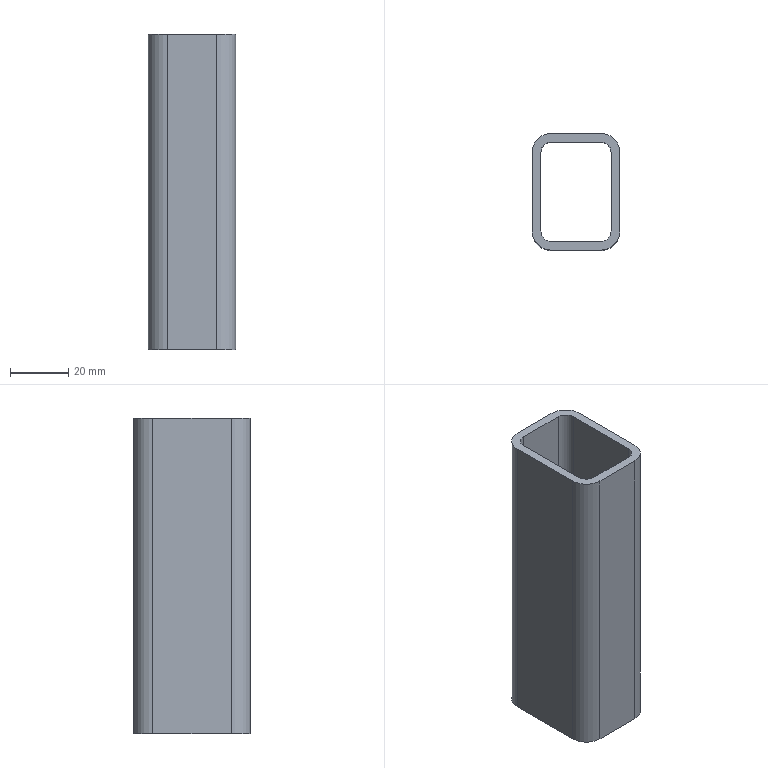Part | STEP file | DIN EN 10305-5 40 x 30 x 3 1785429742031 | 1 solid | 18 faces | box 30 x 40 x 108 mm | volume 38635 mm3 | plane 10 | cylinder 8 | commonest cylinder face diameters 7.2 x4 13.2 x4
STEP:
#1=CARTESIAN_POINT('',(-8.4,-17.,108.));
#2=VERTEX_POINT('',#1);
#3=CARTESIAN_POINT('',(8.4,-17.,108.));
#4=VERTEX_POINT('',#3);
#5=CARTESIAN_POINT('',(4.2,-17.,108.));
#6=DIRECTION('',(1.,0.,0.));
#7=VECTOR('',#6,10.);
#8=LINE('',#5,#7);
#9=EDGE_CURVE('',#2,#4,#8,.T.);
#10=ORIENTED_EDGE('',*,*,#9,.T.);
#11=CARTESIAN_POINT('',(8.4,-17.,0.));
#12=VERTEX_POINT('',#11);
#13=CARTESIAN_POINT('',(8.4,-17.,0.));
#14=DIRECTION('',(0.,0.,1.));
#15=VECTOR('',#14,10.);
#16=LINE('',#13,#15);
#17=EDGE_CURVE('',#12,#4,#16,.T.);
#18=ORIENTED_EDGE('',*,*,#17,.F.);
#19=CARTESIAN_POINT('',(-8.4,-17.,0.));
#20=VERTEX_POINT('',#19);
#21=CARTESIAN_POINT('',(4.2,-17.,0.));
#22=DIRECTION('',(1.,0.,0.));
#23=VECTOR('',#22,10.);
#24=LINE('',#21,#23);
#25=EDGE_CURVE('',#20,#12,#24,.T.);
#26=ORIENTED_EDGE('',*,*,#25,.F.);
#27=CARTESIAN_POINT('',(-8.4,-17.,0.));
#28=DIRECTION('',(0.,0.,1.));
#29=VECTOR('',#28,10.);
#30=LINE('',#27,#29);
#31=EDGE_CURVE('',#20,#2,#30,.T.);
#32=ORIENTED_EDGE('',*,*,#31,.T.);
#33=EDGE_LOOP('',(#10,#18,#26,#32));
#34=FACE_OUTER_BOUND('',#33,.T.);
#35=CARTESIAN_POINT('',(8.4,-17.,0.));
#36=DIRECTION('',(0.,-1.,0.));
#37=DIRECTION('',(0.,0.,-1.));
#38=AXIS2_PLACEMENT_3D('',#35,#36,#37);
#39=PLANE('',#38);
#40=ADVANCED_FACE('',(#34),#39,.F.);
#41=CARTESIAN_POINT('',(12.,-13.4,108.));
#42=VERTEX_POINT('',#41);
#43=CARTESIAN_POINT('',(8.4,-13.4,108.));
#44=DIRECTION('',(0.,0.,1.));
#45=DIRECTION('',(0.,1.,0.));
#46=AXIS2_PLACEMENT_3D('',#43,#44,#45);
#47=CIRCLE('',#46,3.6);
#48=EDGE_CURVE('',#4,#42,#47,.T.);
#49=ORIENTED_EDGE('',*,*,#48,.T.);
#50=CARTESIAN_POINT('',(12.,-13.4,0.));
#51=VERTEX_POINT('',#50);
#52=CARTESIAN_POINT('',(12.,-13.4,0.));
#53=DIRECTION('',(0.,0.,1.));
#54=VECTOR('',#53,10.);
#55=LINE('',#52,#54);
#56=EDGE_CURVE('',#51,#42,#55,.T.);
#57=ORIENTED_EDGE('',*,*,#56,.F.);
#58=CARTESIAN_POINT('',(8.4,-13.4,0.));
#59=DIRECTION('',(0.,0.,1.));
#60=DIRECTION('',(0.,1.,0.));
#61=AXIS2_PLACEMENT_3D('',#58,#59,#60);
#62=CIRCLE('',#61,3.6);
#63=EDGE_CURVE('',#12,#51,#62,.T.);
#64=ORIENTED_EDGE('',*,*,#63,.F.);
#65=ORIENTED_EDGE('',*,*,#17,.T.);
#66=EDGE_LOOP('',(#49,#57,#64,#65));
#67=FACE_OUTER_BOUND('',#66,.T.);
#68=CARTESIAN_POINT('',(8.4,-13.4,0.));
#69=DIRECTION('',(0.,0.,1.));
#70=DIRECTION('',(0.,1.,0.));
#71=AXIS2_PLACEMENT_3D('',#68,#69,#70);
#72=CYLINDRICAL_SURFACE('',#71,3.6);
#73=ADVANCED_FACE('',(#67),#72,.F.);
#74=CARTESIAN_POINT('',(12.,13.4,108.));
#75=VERTEX_POINT('',#74);
#76=CARTESIAN_POINT('',(12.,6.7,108.));
#77=DIRECTION('',(0.,1.,0.));
#78=VECTOR('',#77,10.);
#79=LINE('',#76,#78);
#80=EDGE_CURVE('',#42,#75,#79,.T.);
#81=ORIENTED_EDGE('',*,*,#80,.T.);
#82=CARTESIAN_POINT('',(12.,13.4,0.));
#83=VERTEX_POINT('',#82);
#84=CARTESIAN_POINT('',(12.,13.4,0.));
#85=DIRECTION('',(0.,0.,1.));
#86=VECTOR('',#85,10.);
#87=LINE('',#84,#86);
#88=EDGE_CURVE('',#83,#75,#87,.T.);
#89=ORIENTED_EDGE('',*,*,#88,.F.);
#90=CARTESIAN_POINT('',(12.,6.7,0.));
#91=DIRECTION('',(0.,1.,0.));
#92=VECTOR('',#91,10.);
#93=LINE('',#90,#92);
#94=EDGE_CURVE('',#51,#83,#93,.T.);
#95=ORIENTED_EDGE('',*,*,#94,.F.);
#96=ORIENTED_EDGE('',*,*,#56,.T.);
#97=EDGE_LOOP('',(#81,#89,#95,#96));
#98=FACE_OUTER_BOUND('',#97,.T.);
#99=CARTESIAN_POINT('',(12.,13.4,0.));
#100=DIRECTION('',(1.,0.,0.));
#101=DIRECTION('',(0.,0.,-1.));
#102=AXIS2_PLACEMENT_3D('',#99,#100,#101);
#103=PLANE('',#102);
#104=ADVANCED_FACE('',(#98),#103,.F.);
#105=CARTESIAN_POINT('',(8.4,17.,108.));
#106=VERTEX_POINT('',#105);
#107=CARTESIAN_POINT('',(8.4,13.4,108.));
#108=DIRECTION('',(0.,0.,1.));
#109=DIRECTION('',(-1.,0.,0.));
#110=AXIS2_PLACEMENT_3D('',#107,#108,#109);
#111=CIRCLE('',#110,3.6);
#112=EDGE_CURVE('',#75,#106,#111,.T.);
#113=ORIENTED_EDGE('',*,*,#112,.T.);
#114=CARTESIAN_POINT('',(8.4,17.,0.));
#115=VERTEX_POINT('',#114);
#116=CARTESIAN_POINT('',(8.4,17.,0.));
#117=DIRECTION('',(0.,0.,1.));
#118=VECTOR('',#117,10.);
#119=LINE('',#116,#118);
#120=EDGE_CURVE('',#115,#106,#119,.T.);
#121=ORIENTED_EDGE('',*,*,#120,.F.);
#122=CARTESIAN_POINT('',(8.4,13.4,0.));
#123=DIRECTION('',(0.,0.,1.));
#124=DIRECTION('',(-1.,0.,0.));
#125=AXIS2_PLACEMENT_3D('',#122,#123,#124);
#126=CIRCLE('',#125,3.6);
#127=EDGE_CURVE('',#83,#115,#126,.T.);
#128=ORIENTED_EDGE('',*,*,#127,.F.);
#129=ORIENTED_EDGE('',*,*,#88,.T.);
#130=EDGE_LOOP('',(#113,#121,#128,#129));
#131=FACE_OUTER_BOUND('',#130,.T.);
#132=CARTESIAN_POINT('',(8.4,13.4,0.));
#133=DIRECTION('',(0.,0.,1.));
#134=DIRECTION('',(-1.,0.,0.));
#135=AXIS2_PLACEMENT_3D('',#132,#133,#134);
#136=CYLINDRICAL_SURFACE('',#135,3.6);
#137=ADVANCED_FACE('',(#131),#136,.F.);
#138=CARTESIAN_POINT('',(15.,13.4,108.));
#139=VERTEX_POINT('',#138);
#140=CARTESIAN_POINT('',(15.,-13.4,108.));
#141=VERTEX_POINT('',#140);
#142=CARTESIAN_POINT('',(15.,6.7,108.));
#143=DIRECTION('',(0.,-1.,0.));
#144=VECTOR('',#143,10.);
#145=LINE('',#142,#144);
#146=EDGE_CURVE('',#139,#141,#145,.T.);
#147=ORIENTED_EDGE('',*,*,#146,.T.);
#148=CARTESIAN_POINT('',(15.,-13.4,0.));
#149=VERTEX_POINT('',#148);
#150=CARTESIAN_POINT('',(15.,-13.4,0.));
#151=DIRECTION('',(0.,0.,1.));
#152=VECTOR('',#151,10.);
#153=LINE('',#150,#152);
#154=EDGE_CURVE('',#149,#141,#153,.T.);
#155=ORIENTED_EDGE('',*,*,#154,.F.);
#156=CARTESIAN_POINT('',(15.,13.4,0.));
#157=VERTEX_POINT('',#156);
#158=CARTESIAN_POINT('',(15.,6.7,0.));
#159=DIRECTION('',(0.,-1.,0.));
#160=VECTOR('',#159,10.);
#161=LINE('',#158,#160);
#162=EDGE_CURVE('',#157,#149,#161,.T.);
#163=ORIENTED_EDGE('',*,*,#162,.F.);
#164=CARTESIAN_POINT('',(15.,13.4,0.));
#165=DIRECTION('',(0.,0.,1.));
#166=VECTOR('',#165,10.);
#167=LINE('',#164,#166);
#168=EDGE_CURVE('',#157,#139,#167,.T.);
#169=ORIENTED_EDGE('',*,*,#168,.T.);
#170=EDGE_LOOP('',(#147,#155,#163,#169));
#171=FACE_OUTER_BOUND('',#170,.T.);
#172=CARTESIAN_POINT('',(15.,13.4,0.));
#173=DIRECTION('',(1.,0.,0.));
#174=DIRECTION('',(0.,0.,-1.));
#175=AXIS2_PLACEMENT_3D('',#172,#173,#174);
#176=PLANE('',#175);
#177=ADVANCED_FACE('',(#171),#176,.T.);
#178=CARTESIAN_POINT('',(8.4,-20.,108.));
#179=VERTEX_POINT('',#178);
#180=CARTESIAN_POINT('',(8.4,-13.4,108.));
#181=DIRECTION('',(0.,0.,-1.));
#182=DIRECTION('',(0.,1.,0.));
#183=AXIS2_PLACEMENT_3D('',#180,#181,#182);
#184=CIRCLE('',#183,6.6);
#185=EDGE_CURVE('',#141,#179,#184,.T.);
#186=ORIENTED_EDGE('',*,*,#185,.T.);
#187=CARTESIAN_POINT('',(8.4,-20.,0.));
#188=VERTEX_POINT('',#187);
#189=CARTESIAN_POINT('',(8.4,-20.,0.));
#190=DIRECTION('',(0.,0.,1.));
#191=VECTOR('',#190,10.);
#192=LINE('',#189,#191);
#193=EDGE_CURVE('',#188,#179,#192,.T.);
#194=ORIENTED_EDGE('',*,*,#193,.F.);
#195=CARTESIAN_POINT('',(8.4,-13.4,0.));
#196=DIRECTION('',(0.,0.,-1.));
#197=DIRECTION('',(0.,1.,0.));
#198=AXIS2_PLACEMENT_3D('',#195,#196,#197);
#199=CIRCLE('',#198,6.6);
#200=EDGE_CURVE('',#149,#188,#199,.T.);
#201=ORIENTED_EDGE('',*,*,#200,.F.);
#202=ORIENTED_EDGE('',*,*,#154,.T.);
#203=EDGE_LOOP('',(#186,#194,#201,#202));
#204=FACE_OUTER_BOUND('',#203,.T.);
#205=CARTESIAN_POINT('',(8.4,-13.4,0.));
#206=DIRECTION('',(0.,0.,1.));
#207=DIRECTION('',(0.,1.,0.));
#208=AXIS2_PLACEMENT_3D('',#205,#206,#207);
#209=CYLINDRICAL_SURFACE('',#208,6.6);
#210=ADVANCED_FACE('',(#204),#209,.T.);
#211=CARTESIAN_POINT('',(-8.4,-20.,108.));
#212=VERTEX_POINT('',#211);
#213=CARTESIAN_POINT('',(4.2,-20.,108.));
#214=DIRECTION('',(-1.,0.,0.));
#215=VECTOR('',#214,10.);
#216=LINE('',#213,#215);
#217=EDGE_CURVE('',#179,#212,#216,.T.);
#218=ORIENTED_EDGE('',*,*,#217,.T.);
#219=CARTESIAN_POINT('',(-8.4,-20.,0.));
#220=VERTEX_POINT('',#219);
#221=CARTESIAN_POINT('',(-8.4,-20.,0.));
#222=DIRECTION('',(0.,0.,1.));
#223=VECTOR('',#222,10.);
#224=LINE('',#221,#223);
#225=EDGE_CURVE('',#220,#212,#224,.T.);
#226=ORIENTED_EDGE('',*,*,#225,.F.);
#227=CARTESIAN_POINT('',(4.2,-20.,0.));
#228=DIRECTION('',(-1.,0.,0.));
#229=VECTOR('',#228,10.);
#230=LINE('',#227,#229);
#231=EDGE_CURVE('',#188,#220,#230,.T.);
#232=ORIENTED_EDGE('',*,*,#231,.F.);
#233=ORIENTED_EDGE('',*,*,#193,.T.);
#234=EDGE_LOOP('',(#218,#226,#232,#233));
#235=FACE_OUTER_BOUND('',#234,.T.);
#236=CARTESIAN_POINT('',(8.4,-20.,0.));
#237=DIRECTION('',(0.,-1.,0.));
#238=DIRECTION('',(0.,0.,-1.));
#239=AXIS2_PLACEMENT_3D('',#236,#237,#238);
#240=PLANE('',#239);
#241=ADVANCED_FACE('',(#235),#240,.T.);
#242=CARTESIAN_POINT('',(-15.,-13.4,108.));
#243=VERTEX_POINT('',#242);
#244=CARTESIAN_POINT('',(-8.4,-13.4,108.));
#245=DIRECTION('',(0.,0.,-1.));
#246=DIRECTION('',(1.,0.,0.));
#247=AXIS2_PLACEMENT_3D('',#244,#245,#246);
#248=CIRCLE('',#247,6.6);
#249=EDGE_CURVE('',#212,#243,#248,.T.);
#250=ORIENTED_EDGE('',*,*,#249,.T.);
#251=CARTESIAN_POINT('',(-15.,-13.4,0.));
#252=VERTEX_POINT('',#251);
#253=CARTESIAN_POINT('',(-15.,-13.4,0.));
#254=DIRECTION('',(0.,0.,1.));
#255=VECTOR('',#254,10.);
#256=LINE('',#253,#255);
#257=EDGE_CURVE('',#252,#243,#256,.T.);
#258=ORIENTED_EDGE('',*,*,#257,.F.);
#259=CARTESIAN_POINT('',(-8.4,-13.4,0.));
#260=DIRECTION('',(0.,0.,-1.));
#261=DIRECTION('',(1.,0.,0.));
#262=AXIS2_PLACEMENT_3D('',#259,#260,#261);
#263=CIRCLE('',#262,6.6);
#264=EDGE_CURVE('',#220,#252,#263,.T.);
#265=ORIENTED_EDGE('',*,*,#264,.F.);
#266=ORIENTED_EDGE('',*,*,#225,.T.);
#267=EDGE_LOOP('',(#250,#258,#265,#266));
#268=FACE_OUTER_BOUND('',#267,.T.);
#269=CARTESIAN_POINT('',(-8.4,-13.4,0.));
#270=DIRECTION('',(0.,0.,1.));
#271=DIRECTION('',(1.,0.,0.));
#272=AXIS2_PLACEMENT_3D('',#269,#270,#271);
#273=CYLINDRICAL_SURFACE('',#272,6.6);
#274=ADVANCED_FACE('',(#268),#273,.T.);
#275=CARTESIAN_POINT('',(-8.4,17.,108.));
#276=VERTEX_POINT('',#275);
#277=CARTESIAN_POINT('',(-4.2,17.,108.));
#278=DIRECTION('',(-1.,0.,0.));
#279=VECTOR('',#278,10.);
#280=LINE('',#277,#279);
#281=EDGE_CURVE('',#106,#276,#280,.T.);
#282=ORIENTED_EDGE('',*,*,#281,.T.);
#283=CARTESIAN_POINT('',(-8.4,17.,0.));
#284=VERTEX_POINT('',#283);
#285=CARTESIAN_POINT('',(-8.4,17.,0.));
#286=DIRECTION('',(0.,0.,1.));
#287=VECTOR('',#286,10.);
#288=LINE('',#285,#287);
#289=EDGE_CURVE('',#284,#276,#288,.T.);
#290=ORIENTED_EDGE('',*,*,#289,.F.);
#291=CARTESIAN_POINT('',(-4.2,17.,0.));
#292=DIRECTION('',(-1.,0.,0.));
#293=VECTOR('',#292,10.);
#294=LINE('',#291,#293);
#295=EDGE_CURVE('',#115,#284,#294,.T.);
#296=ORIENTED_EDGE('',*,*,#295,.F.);
#297=ORIENTED_EDGE('',*,*,#120,.T.);
#298=EDGE_LOOP('',(#282,#290,#296,#297));
#299=FACE_OUTER_BOUND('',#298,.T.);
#300=CARTESIAN_POINT('',(-8.4,17.,0.));
#301=DIRECTION('',(0.,1.,0.));
#302=DIRECTION('',(0.,0.,1.));
#303=AXIS2_PLACEMENT_3D('',#300,#301,#302);
#304=PLANE('',#303);
#305=ADVANCED_FACE('',(#299),#304,.F.);
#306=CARTESIAN_POINT('',(-12.,-13.4,108.));
#307=VERTEX_POINT('',#306);
#308=CARTESIAN_POINT('',(-8.4,-13.4,108.));
#309=DIRECTION('',(0.,0.,1.));
#310=DIRECTION('',(1.,0.,0.));
#311=AXIS2_PLACEMENT_3D('',#308,#309,#310);
#312=CIRCLE('',#311,3.6);
#313=EDGE_CURVE('',#307,#2,#312,.T.);
#314=ORIENTED_EDGE('',*,*,#313,.T.);
#315=ORIENTED_EDGE('',*,*,#31,.F.);
#316=CARTESIAN_POINT('',(-12.,-13.4,0.));
#317=VERTEX_POINT('',#316);
#318=CARTESIAN_POINT('',(-8.4,-13.4,0.));
#319=DIRECTION('',(0.,0.,1.));
#320=DIRECTION('',(1.,0.,0.));
#321=AXIS2_PLACEMENT_3D('',#318,#319,#320);
#322=CIRCLE('',#321,3.6);
#323=EDGE_CURVE('',#317,#20,#322,.T.);
#324=ORIENTED_EDGE('',*,*,#323,.F.);
#325=CARTESIAN_POINT('',(-12.,-13.4,0.));
#326=DIRECTION('',(0.,0.,1.));
#327=VECTOR('',#326,10.);
#328=LINE('',#325,#327);
#329=EDGE_CURVE('',#317,#307,#328,.T.);
#330=ORIENTED_EDGE('',*,*,#329,.T.);
#331=EDGE_LOOP('',(#314,#315,#324,#330));
#332=FACE_OUTER_BOUND('',#331,.T.);
#333=CARTESIAN_POINT('',(-8.4,-13.4,0.));
#334=DIRECTION('',(0.,0.,1.));
#335=DIRECTION('',(1.,0.,0.));
#336=AXIS2_PLACEMENT_3D('',#333,#334,#335);
#337=CYLINDRICAL_SURFACE('',#336,3.6);
#338=ADVANCED_FACE('',(#332),#337,.F.);
#339=CARTESIAN_POINT('',(-12.,13.4,108.));
#340=VERTEX_POINT('',#339);
#341=CARTESIAN_POINT('',(-12.,-6.7,108.));
#342=DIRECTION('',(0.,-1.,0.));
#343=VECTOR('',#342,10.);
#344=LINE('',#341,#343);
#345=EDGE_CURVE('',#340,#307,#344,.T.);
#346=ORIENTED_EDGE('',*,*,#345,.T.);
#347=ORIENTED_EDGE('',*,*,#329,.F.);
#348=CARTESIAN_POINT('',(-12.,13.4,0.));
#349=VERTEX_POINT('',#348);
#350=CARTESIAN_POINT('',(-12.,-6.7,0.));
#351=DIRECTION('',(0.,-1.,0.));
#352=VECTOR('',#351,10.);
#353=LINE('',#350,#352);
#354=EDGE_CURVE('',#349,#317,#353,.T.);
#355=ORIENTED_EDGE('',*,*,#354,.F.);
#356=CARTESIAN_POINT('',(-12.,13.4,0.));
#357=DIRECTION('',(0.,0.,1.));
#358=VECTOR('',#357,10.);
#359=LINE('',#356,#358);
#360=EDGE_CURVE('',#349,#340,#359,.T.);
#361=ORIENTED_EDGE('',*,*,#360,.T.);
#362=EDGE_LOOP('',(#346,#347,#355,#361));
#363=FACE_OUTER_BOUND('',#362,.T.);
#364=CARTESIAN_POINT('',(-12.,-13.4,0.));
#365=DIRECTION('',(-1.,0.,0.));
#366=DIRECTION('',(0.,0.,1.));
#367=AXIS2_PLACEMENT_3D('',#364,#365,#366);
#368=PLANE('',#367);
#369=ADVANCED_FACE('',(#363),#368,.F.);
#370=CARTESIAN_POINT('',(-8.4,13.4,108.));
#371=DIRECTION('',(0.,0.,1.));
#372=DIRECTION('',(0.,-1.,0.));
#373=AXIS2_PLACEMENT_3D('',#370,#371,#372);
#374=CIRCLE('',#373,3.6);
#375=EDGE_CURVE('',#276,#340,#374,.T.);
#376=ORIENTED_EDGE('',*,*,#375,.T.);
#377=ORIENTED_EDGE('',*,*,#360,.F.);
#378=CARTESIAN_POINT('',(-8.4,13.4,0.));
#379=DIRECTION('',(0.,0.,1.));
#380=DIRECTION('',(0.,-1.,0.));
#381=AXIS2_PLACEMENT_3D('',#378,#379,#380);
#382=CIRCLE('',#381,3.6);
#383=EDGE_CURVE('',#284,#349,#382,.T.);
#384=ORIENTED_EDGE('',*,*,#383,.F.);
#385=ORIENTED_EDGE('',*,*,#289,.T.);
#386=EDGE_LOOP('',(#376,#377,#384,#385));
#387=FACE_OUTER_BOUND('',#386,.T.);
#388=CARTESIAN_POINT('',(-8.4,13.4,0.));
#389=DIRECTION('',(0.,0.,1.));
#390=DIRECTION('',(0.,-1.,0.));
#391=AXIS2_PLACEMENT_3D('',#388,#389,#390);
#392=CYLINDRICAL_SURFACE('',#391,3.6);
#393=ADVANCED_FACE('',(#387),#392,.F.);
#394=CARTESIAN_POINT('',(-15.,13.4,108.));
#395=VERTEX_POINT('',#394);
#396=CARTESIAN_POINT('',(-15.,-6.7,108.));
#397=DIRECTION('',(0.,1.,0.));
#398=VECTOR('',#397,10.);
#399=LINE('',#396,#398);
#400=EDGE_CURVE('',#243,#395,#399,.T.);
#401=ORIENTED_EDGE('',*,*,#400,.T.);
#402=CARTESIAN_POINT('',(-15.,13.4,0.));
#403=VERTEX_POINT('',#402);
#404=CARTESIAN_POINT('',(-15.,13.4,0.));
#405=DIRECTION('',(0.,0.,1.));
#406=VECTOR('',#405,10.);
#407=LINE('',#404,#406);
#408=EDGE_CURVE('',#403,#395,#407,.T.);
#409=ORIENTED_EDGE('',*,*,#408,.F.);
#410=CARTESIAN_POINT('',(-15.,-6.7,0.));
#411=DIRECTION('',(0.,1.,0.));
#412=VECTOR('',#411,10.);
#413=LINE('',#410,#412);
#414=EDGE_CURVE('',#252,#403,#413,.T.);
#415=ORIENTED_EDGE('',*,*,#414,.F.);
#416=ORIENTED_EDGE('',*,*,#257,.T.);
#417=EDGE_LOOP('',(#401,#409,#415,#416));
#418=FACE_OUTER_BOUND('',#417,.T.);
#419=CARTESIAN_POINT('',(-15.,-13.4,0.));
#420=DIRECTION('',(-1.,0.,0.));
#421=DIRECTION('',(0.,0.,1.));
#422=AXIS2_PLACEMENT_3D('',#419,#420,#421);
#423=PLANE('',#422);
#424=ADVANCED_FACE('',(#418),#423,.T.);
#425=CARTESIAN_POINT('',(-8.4,20.,108.));
#426=VERTEX_POINT('',#425);
#427=CARTESIAN_POINT('',(-8.4,13.4,108.));
#428=DIRECTION('',(0.,0.,-1.));
#429=DIRECTION('',(0.,-1.,0.));
#430=AXIS2_PLACEMENT_3D('',#427,#428,#429);
#431=CIRCLE('',#430,6.6);
#432=EDGE_CURVE('',#395,#426,#431,.T.);
#433=ORIENTED_EDGE('',*,*,#432,.T.);
#434=CARTESIAN_POINT('',(-8.4,20.,0.));
#435=VERTEX_POINT('',#434);
#436=CARTESIAN_POINT('',(-8.4,20.,0.));
#437=DIRECTION('',(0.,0.,1.));
#438=VECTOR('',#437,10.);
#439=LINE('',#436,#438);
#440=EDGE_CURVE('',#435,#426,#439,.T.);
#441=ORIENTED_EDGE('',*,*,#440,.F.);
#442=CARTESIAN_POINT('',(-8.4,13.4,0.));
#443=DIRECTION('',(0.,0.,-1.));
#444=DIRECTION('',(0.,-1.,0.));
#445=AXIS2_PLACEMENT_3D('',#442,#443,#444);
#446=CIRCLE('',#445,6.6);
#447=EDGE_CURVE('',#403,#435,#446,.T.);
#448=ORIENTED_EDGE('',*,*,#447,.F.);
#449=ORIENTED_EDGE('',*,*,#408,.T.);
#450=EDGE_LOOP('',(#433,#441,#448,#449));
#451=FACE_OUTER_BOUND('',#450,.T.);
#452=CARTESIAN_POINT('',(-8.4,13.4,0.));
#453=DIRECTION('',(0.,0.,1.));
#454=DIRECTION('',(0.,-1.,0.));
#455=AXIS2_PLACEMENT_3D('',#452,#453,#454);
#456=CYLINDRICAL_SURFACE('',#455,6.6);
#457=ADVANCED_FACE('',(#451),#456,.T.);
#458=CARTESIAN_POINT('',(8.4,20.,108.));
#459=VERTEX_POINT('',#458);
#460=CARTESIAN_POINT('',(-4.2,20.,108.));
#461=DIRECTION('',(1.,0.,0.));
#462=VECTOR('',#461,10.);
#463=LINE('',#460,#462);
#464=EDGE_CURVE('',#426,#459,#463,.T.);
#465=ORIENTED_EDGE('',*,*,#464,.T.);
#466=CARTESIAN_POINT('',(8.4,20.,0.));
#467=VERTEX_POINT('',#466);
#468=CARTESIAN_POINT('',(8.4,20.,0.));
#469=DIRECTION('',(0.,0.,1.));
#470=VECTOR('',#469,10.);
#471=LINE('',#468,#470);
#472=EDGE_CURVE('',#467,#459,#471,.T.);
#473=ORIENTED_EDGE('',*,*,#472,.F.);
#474=CARTESIAN_POINT('',(-4.2,20.,0.));
#475=DIRECTION('',(1.,0.,0.));
#476=VECTOR('',#475,10.);
#477=LINE('',#474,#476);
#478=EDGE_CURVE('',#435,#467,#477,.T.);
#479=ORIENTED_EDGE('',*,*,#478,.F.);
#480=ORIENTED_EDGE('',*,*,#440,.T.);
#481=EDGE_LOOP('',(#465,#473,#479,#480));
#482=FACE_OUTER_BOUND('',#481,.T.);
#483=CARTESIAN_POINT('',(-8.4,20.,0.));
#484=DIRECTION('',(0.,1.,0.));
#485=DIRECTION('',(0.,0.,1.));
#486=AXIS2_PLACEMENT_3D('',#483,#484,#485);
#487=PLANE('',#486);
#488=ADVANCED_FACE('',(#482),#487,.T.);
#489=CARTESIAN_POINT('',(8.4,13.4,108.));
#490=DIRECTION('',(0.,0.,-1.));
#491=DIRECTION('',(-1.,0.,0.));
#492=AXIS2_PLACEMENT_3D('',#489,#490,#491);
#493=CIRCLE('',#492,6.6);
#494=EDGE_CURVE('',#459,#139,#493,.T.);
#495=ORIENTED_EDGE('',*,*,#494,.T.);
#496=ORIENTED_EDGE('',*,*,#168,.F.);
#497=CARTESIAN_POINT('',(8.4,13.4,0.));
#498=DIRECTION('',(0.,0.,-1.));
#499=DIRECTION('',(-1.,0.,0.));
#500=AXIS2_PLACEMENT_3D('',#497,#498,#499);
#501=CIRCLE('',#500,6.6);
#502=EDGE_CURVE('',#467,#157,#501,.T.);
#503=ORIENTED_EDGE('',*,*,#502,.F.);
#504=ORIENTED_EDGE('',*,*,#472,.T.);
#505=EDGE_LOOP('',(#495,#496,#503,#504));
#506=FACE_OUTER_BOUND('',#505,.T.);
#507=CARTESIAN_POINT('',(8.4,13.4,0.));
#508=DIRECTION('',(0.,0.,1.));
#509=DIRECTION('',(-1.,0.,0.));
#510=AXIS2_PLACEMENT_3D('',#507,#508,#509);
#511=CYLINDRICAL_SURFACE('',#510,6.6);
#512=ADVANCED_FACE('',(#506),#511,.T.);
#513=ORIENTED_EDGE('',*,*,#414,.T.);
#514=ORIENTED_EDGE('',*,*,#447,.T.);
#515=ORIENTED_EDGE('',*,*,#478,.T.);
#516=ORIENTED_EDGE('',*,*,#502,.T.);
#517=ORIENTED_EDGE('',*,*,#162,.T.);
#518=ORIENTED_EDGE('',*,*,#200,.T.);
#519=ORIENTED_EDGE('',*,*,#231,.T.);
#520=ORIENTED_EDGE('',*,*,#264,.T.);
#521=EDGE_LOOP('',(#513,#514,#515,#516,#517,#518,#519,#520));
#522=FACE_OUTER_BOUND('',#521,.T.);
#523=ORIENTED_EDGE('',*,*,#295,.T.);
#524=ORIENTED_EDGE('',*,*,#383,.T.);
#525=ORIENTED_EDGE('',*,*,#354,.T.);
#526=ORIENTED_EDGE('',*,*,#323,.T.);
#527=ORIENTED_EDGE('',*,*,#25,.T.);
#528=ORIENTED_EDGE('',*,*,#63,.T.);
#529=ORIENTED_EDGE('',*,*,#94,.T.);
#530=ORIENTED_EDGE('',*,*,#127,.T.);
#531=EDGE_LOOP('',(#523,#524,#525,#526,#527,#528,#529,#530));
#532=FACE_BOUND('',#531,.T.);
#533=CARTESIAN_POINT('',(0.,0.,0.));
#534=DIRECTION('',(0.,0.,1.));
#535=DIRECTION('',(1.,0.,0.));
#536=AXIS2_PLACEMENT_3D('',#533,#534,#535);
#537=PLANE('',#536);
#538=ADVANCED_FACE('',(#522,#532),#537,.F.);
#539=ORIENTED_EDGE('',*,*,#400,.F.);
#540=ORIENTED_EDGE('',*,*,#249,.F.);
#541=ORIENTED_EDGE('',*,*,#217,.F.);
#542=ORIENTED_EDGE('',*,*,#185,.F.);
#543=ORIENTED_EDGE('',*,*,#146,.F.);
#544=ORIENTED_EDGE('',*,*,#494,.F.);
#545=ORIENTED_EDGE('',*,*,#464,.F.);
#546=ORIENTED_EDGE('',*,*,#432,.F.);
#547=EDGE_LOOP('',(#539,#540,#541,#542,#543,#544,#545,#546));
#548=FACE_OUTER_BOUND('',#547,.T.);
#549=ORIENTED_EDGE('',*,*,#281,.F.);
#550=ORIENTED_EDGE('',*,*,#112,.F.);
#551=ORIENTED_EDGE('',*,*,#80,.F.);
#552=ORIENTED_EDGE('',*,*,#48,.F.);
#553=ORIENTED_EDGE('',*,*,#9,.F.);
#554=ORIENTED_EDGE('',*,*,#313,.F.);
#555=ORIENTED_EDGE('',*,*,#345,.F.);
#556=ORIENTED_EDGE('',*,*,#375,.F.);
#557=EDGE_LOOP('',(#549,#550,#551,#552,#553,#554,#555,#556));
#558=FACE_BOUND('',#557,.T.);
#559=CARTESIAN_POINT('',(0.,0.,108.));
#560=DIRECTION('',(0.,0.,1.));
#561=DIRECTION('',(1.,0.,0.));
#562=AXIS2_PLACEMENT_3D('',#559,#560,#561);
#563=PLANE('',#562);
#564=ADVANCED_FACE('',(#548,#558),#563,.T.);
#565=CLOSED_SHELL('',(#40,#73,#104,#137,#177,#210,#241,#274,#305,#338,#369,#393,#424,#457,#488,#512,#538,#564));
#566=MANIFOLD_SOLID_BREP('',#565);
#567=(LENGTH_UNIT()NAMED_UNIT(*)SI_UNIT(.MILLI.,.METRE.));
#568=UNCERTAINTY_MEASURE_WITH_UNIT(LENGTH_MEASURE(0.01),#567,'','');
#569=(NAMED_UNIT(*)PLANE_ANGLE_UNIT()SI_UNIT($,.RADIAN.));
#570=(NAMED_UNIT(*)SI_UNIT($,.STERADIAN.)SOLID_ANGLE_UNIT());
#571=(GEOMETRIC_REPRESENTATION_CONTEXT(3)GLOBAL_UNCERTAINTY_ASSIGNED_CONTEXT((#568))GLOBAL_UNIT_ASSIGNED_CONTEXT((#567,#569,#570))REPRESENTATION_CONTEXT('',''));
#572=ADVANCED_BREP_SHAPE_REPRESENTATION('',(#566),#571);